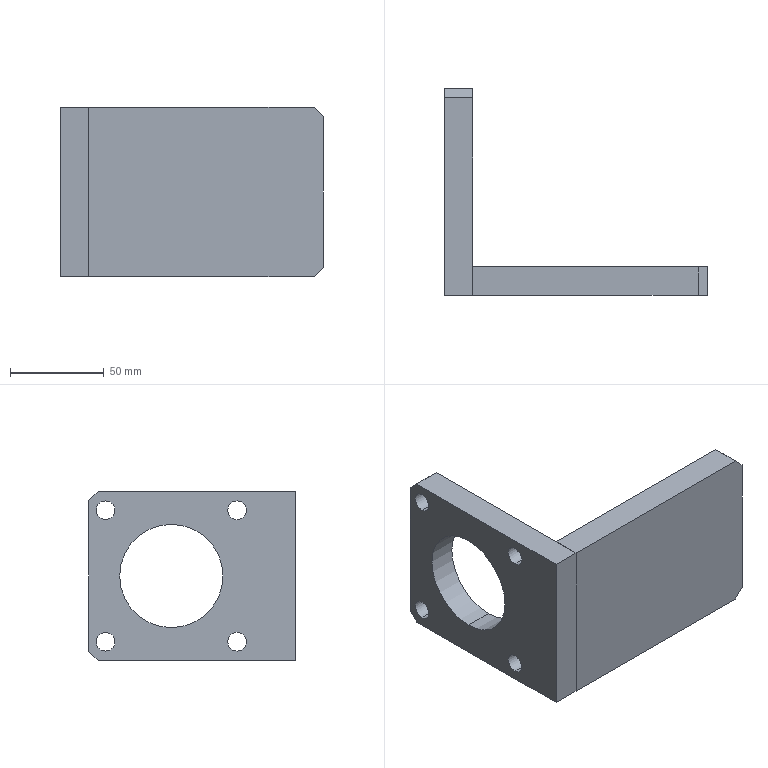Part | STEP file | Hydraulic Cylinder Fixing Bracket | 2 solids | 46 faces | box 140 x 110 x 90 mm | volume 268205 mm3 | plane 28 | cylinder 18 | commonest cylinder face diameters 9 x8 10 x8 55 x2
STEP:
#1=CARTESIAN_POINT('',(-38.428,-20.407,0.));
#2=VERTEX_POINT('',#1);
#3=CARTESIAN_POINT('',(81.572,-20.407,0.));
#4=VERTEX_POINT('',#3);
#5=CARTESIAN_POINT('',(-38.428,-20.407,0.));
#6=DIRECTION('',(1.,0.,0.));
#7=VECTOR('',#6,1000.);
#8=LINE('',#5,#7);
#9=EDGE_CURVE('',#2,#4,#8,.T.);
#10=ORIENTED_EDGE('',*,*,#9,.T.);
#11=CARTESIAN_POINT('',(86.572,-20.407,5.));
#12=VERTEX_POINT('',#11);
#13=CARTESIAN_POINT('',(81.572,-20.407,0.));
#14=DIRECTION('',(0.7071,0.,0.7071));
#15=VECTOR('',#14,1000.);
#16=LINE('',#13,#15);
#17=EDGE_CURVE('',#4,#12,#16,.T.);
#18=ORIENTED_EDGE('',*,*,#17,.T.);
#19=CARTESIAN_POINT('',(86.572,-20.407,85.));
#20=VERTEX_POINT('',#19);
#21=CARTESIAN_POINT('',(86.572,-20.407,-125.897));
#22=DIRECTION('',(0.,0.,1.));
#23=VECTOR('',#22,1000.);
#24=LINE('',#21,#23);
#25=EDGE_CURVE('',#12,#20,#24,.T.);
#26=ORIENTED_EDGE('',*,*,#25,.T.);
#27=CARTESIAN_POINT('',(81.572,-20.407,90.));
#28=VERTEX_POINT('',#27);
#29=CARTESIAN_POINT('',(86.572,-20.407,85.));
#30=DIRECTION('',(-0.7071,0.,0.7071));
#31=VECTOR('',#30,1000.);
#32=LINE('',#29,#31);
#33=EDGE_CURVE('',#20,#28,#32,.T.);
#34=ORIENTED_EDGE('',*,*,#33,.T.);
#35=CARTESIAN_POINT('',(-38.428,-20.407,90.));
#36=VERTEX_POINT('',#35);
#37=CARTESIAN_POINT('',(-38.428,-20.407,90.));
#38=DIRECTION('',(-1.,0.,0.));
#39=VECTOR('',#38,1000.);
#40=LINE('',#37,#39);
#41=EDGE_CURVE('',#28,#36,#40,.T.);
#42=ORIENTED_EDGE('',*,*,#41,.T.);
#43=CARTESIAN_POINT('',(-38.428,-20.407,-125.897));
#44=DIRECTION('',(0.,0.,-1.));
#45=VECTOR('',#44,1000.);
#46=LINE('',#43,#45);
#47=EDGE_CURVE('',#36,#2,#46,.T.);
#48=ORIENTED_EDGE('',*,*,#47,.T.);
#49=EDGE_LOOP('',(#10,#18,#26,#34,#42,#48));
#50=FACE_OUTER_BOUND('',#49,.T.);
#51=CARTESIAN_POINT('',(-38.428,-20.407,-125.897));
#52=DIRECTION('',(0.,-1.,0.));
#53=DIRECTION('',(0.,0.,-1.));
#54=AXIS2_PLACEMENT_3D('',#51,#52,#53);
#55=PLANE('',#54);
#56=ADVANCED_FACE('',(#50),#55,.T.);
#57=CARTESIAN_POINT('',(81.572,-5.407,0.));
#58=VERTEX_POINT('',#57);
#59=CARTESIAN_POINT('',(81.572,-20.407,0.));
#60=DIRECTION('',(0.,-1.,0.));
#61=VECTOR('',#60,1000.);
#62=LINE('',#59,#61);
#63=EDGE_CURVE('',#58,#4,#62,.T.);
#64=ORIENTED_EDGE('',*,*,#63,.F.);
#65=CARTESIAN_POINT('',(86.572,-5.407,5.));
#66=VERTEX_POINT('',#65);
#67=CARTESIAN_POINT('',(86.572,-5.407,5.));
#68=DIRECTION('',(-0.7071,0.,-0.7071));
#69=VECTOR('',#68,1000.);
#70=LINE('',#67,#69);
#71=EDGE_CURVE('',#66,#58,#70,.T.);
#72=ORIENTED_EDGE('',*,*,#71,.F.);
#73=CARTESIAN_POINT('',(86.572,-20.407,5.));
#74=DIRECTION('',(0.,1.,0.));
#75=VECTOR('',#74,1000.);
#76=LINE('',#73,#75);
#77=EDGE_CURVE('',#12,#66,#76,.T.);
#78=ORIENTED_EDGE('',*,*,#77,.F.);
#79=ORIENTED_EDGE('',*,*,#17,.F.);
#80=EDGE_LOOP('',(#64,#72,#78,#79));
#81=FACE_OUTER_BOUND('',#80,.T.);
#82=CARTESIAN_POINT('',(86.572,-20.407,5.));
#83=DIRECTION('',(-0.7071,0.,0.7071));
#84=DIRECTION('',(0.7071,0.,0.7071));
#85=AXIS2_PLACEMENT_3D('',#82,#83,#84);
#86=PLANE('',#85);
#87=ADVANCED_FACE('',(#81),#86,.F.);
#88=ORIENTED_EDGE('',*,*,#9,.F.);
#89=CARTESIAN_POINT('',(-38.428,-5.407,0.));
#90=VERTEX_POINT('',#89);
#91=CARTESIAN_POINT('',(-38.428,0.,0.));
#92=DIRECTION('',(0.,1.,0.));
#93=VECTOR('',#92,1000.);
#94=LINE('',#91,#93);
#95=EDGE_CURVE('',#2,#90,#94,.T.);
#96=ORIENTED_EDGE('',*,*,#95,.T.);
#97=CARTESIAN_POINT('',(0.,-5.407,0.));
#98=DIRECTION('',(1.,0.,0.));
#99=VECTOR('',#98,1000.);
#100=LINE('',#97,#99);
#101=EDGE_CURVE('',#90,#58,#100,.T.);
#102=ORIENTED_EDGE('',*,*,#101,.T.);
#103=ORIENTED_EDGE('',*,*,#63,.T.);
#104=EDGE_LOOP('',(#88,#96,#102,#103));
#105=FACE_OUTER_BOUND('',#104,.T.);
#106=CARTESIAN_POINT('',(0.,0.,0.));
#107=DIRECTION('',(0.,0.,-1.));
#108=DIRECTION('',(-1.,0.,0.));
#109=AXIS2_PLACEMENT_3D('',#106,#107,#108);
#110=PLANE('',#109);
#111=ADVANCED_FACE('',(#105),#110,.T.);
#112=ORIENTED_EDGE('',*,*,#47,.F.);
#113=CARTESIAN_POINT('',(-38.428,-5.407,90.));
#114=VERTEX_POINT('',#113);
#115=CARTESIAN_POINT('',(-38.428,-20.407,90.));
#116=DIRECTION('',(0.,1.,0.));
#117=VECTOR('',#116,1000.);
#118=LINE('',#115,#117);
#119=EDGE_CURVE('',#36,#114,#118,.T.);
#120=ORIENTED_EDGE('',*,*,#119,.T.);
#121=CARTESIAN_POINT('',(-38.428,-5.407,-125.897));
#122=DIRECTION('',(0.,0.,-1.));
#123=VECTOR('',#122,1000.);
#124=LINE('',#121,#123);
#125=EDGE_CURVE('',#114,#90,#124,.T.);
#126=ORIENTED_EDGE('',*,*,#125,.T.);
#127=ORIENTED_EDGE('',*,*,#95,.F.);
#128=EDGE_LOOP('',(#112,#120,#126,#127));
#129=FACE_OUTER_BOUND('',#128,.T.);
#130=CARTESIAN_POINT('',(-38.428,-20.407,-125.897));
#131=DIRECTION('',(-1.,0.,0.));
#132=DIRECTION('',(0.,0.,1.));
#133=AXIS2_PLACEMENT_3D('',#130,#131,#132);
#134=PLANE('',#133);
#135=ADVANCED_FACE('',(#129),#134,.T.);
#136=CARTESIAN_POINT('',(81.572,-5.407,90.));
#137=VERTEX_POINT('',#136);
#138=CARTESIAN_POINT('',(81.572,0.,90.));
#139=DIRECTION('',(0.,-1.,0.));
#140=VECTOR('',#139,1000.);
#141=LINE('',#138,#140);
#142=EDGE_CURVE('',#137,#28,#141,.T.);
#143=ORIENTED_EDGE('',*,*,#142,.F.);
#144=CARTESIAN_POINT('',(0.,-5.407,90.));
#145=DIRECTION('',(1.,0.,0.));
#146=VECTOR('',#145,1000.);
#147=LINE('',#144,#146);
#148=EDGE_CURVE('',#114,#137,#147,.T.);
#149=ORIENTED_EDGE('',*,*,#148,.F.);
#150=ORIENTED_EDGE('',*,*,#119,.F.);
#151=ORIENTED_EDGE('',*,*,#41,.F.);
#152=EDGE_LOOP('',(#143,#149,#150,#151));
#153=FACE_OUTER_BOUND('',#152,.T.);
#154=CARTESIAN_POINT('',(0.,0.,90.));
#155=DIRECTION('',(0.,0.,-1.));
#156=DIRECTION('',(-1.,0.,0.));
#157=AXIS2_PLACEMENT_3D('',#154,#155,#156);
#158=PLANE('',#157);
#159=ADVANCED_FACE('',(#153),#158,.F.);
#160=CARTESIAN_POINT('',(86.572,-5.407,85.));
#161=VERTEX_POINT('',#160);
#162=CARTESIAN_POINT('',(81.572,-5.407,90.));
#163=DIRECTION('',(-0.7071,0.,0.7071));
#164=VECTOR('',#163,1000.);
#165=LINE('',#162,#164);
#166=EDGE_CURVE('',#161,#137,#165,.T.);
#167=ORIENTED_EDGE('',*,*,#166,.T.);
#168=ORIENTED_EDGE('',*,*,#142,.T.);
#169=ORIENTED_EDGE('',*,*,#33,.F.);
#170=CARTESIAN_POINT('',(86.572,0.,85.));
#171=DIRECTION('',(0.,1.,0.));
#172=VECTOR('',#171,1000.);
#173=LINE('',#170,#172);
#174=EDGE_CURVE('',#20,#161,#173,.T.);
#175=ORIENTED_EDGE('',*,*,#174,.T.);
#176=EDGE_LOOP('',(#167,#168,#169,#175));
#177=FACE_OUTER_BOUND('',#176,.T.);
#178=CARTESIAN_POINT('',(81.572,0.,90.));
#179=DIRECTION('',(0.7071,0.,0.7071));
#180=DIRECTION('',(0.7071,0.,-0.7071));
#181=AXIS2_PLACEMENT_3D('',#178,#179,#180);
#182=PLANE('',#181);
#183=ADVANCED_FACE('',(#177),#182,.T.);
#184=ORIENTED_EDGE('',*,*,#25,.F.);
#185=ORIENTED_EDGE('',*,*,#77,.T.);
#186=CARTESIAN_POINT('',(86.572,-5.407,-125.897));
#187=DIRECTION('',(0.,0.,1.));
#188=VECTOR('',#187,1000.);
#189=LINE('',#186,#188);
#190=EDGE_CURVE('',#66,#161,#189,.T.);
#191=ORIENTED_EDGE('',*,*,#190,.T.);
#192=ORIENTED_EDGE('',*,*,#174,.F.);
#193=EDGE_LOOP('',(#184,#185,#191,#192));
#194=FACE_OUTER_BOUND('',#193,.T.);
#195=CARTESIAN_POINT('',(86.572,-20.407,-125.897));
#196=DIRECTION('',(1.,0.,0.));
#197=DIRECTION('',(0.,1.,0.));
#198=AXIS2_PLACEMENT_3D('',#195,#196,#197);
#199=PLANE('',#198);
#200=ADVANCED_FACE('',(#194),#199,.T.);
#201=ORIENTED_EDGE('',*,*,#101,.F.);
#202=ORIENTED_EDGE('',*,*,#125,.F.);
#203=ORIENTED_EDGE('',*,*,#148,.T.);
#204=ORIENTED_EDGE('',*,*,#166,.F.);
#205=ORIENTED_EDGE('',*,*,#190,.F.);
#206=ORIENTED_EDGE('',*,*,#71,.T.);
#207=EDGE_LOOP('',(#201,#202,#203,#204,#205,#206));
#208=FACE_OUTER_BOUND('',#207,.T.);
#209=CARTESIAN_POINT('',(19.072,-5.407,7.5));
#210=VERTEX_POINT('',#209);
#211=CARTESIAN_POINT('',(19.072,-5.407,16.5));
#212=VERTEX_POINT('',#211);
#213=CARTESIAN_POINT('',(19.072,-5.407,12.));
#214=DIRECTION('',(0.,-1.,0.));
#215=DIRECTION('',(0.,0.,1.));
#216=AXIS2_PLACEMENT_3D('',#213,#214,#215);
#217=CIRCLE('',#216,4.5);
#218=EDGE_CURVE('',#210,#212,#217,.T.);
#219=ORIENTED_EDGE('',*,*,#218,.T.);
#220=CARTESIAN_POINT('',(4.072,-5.407,16.5));
#221=VERTEX_POINT('',#220);
#222=CARTESIAN_POINT('',(-38.428,-5.407,16.5));
#223=DIRECTION('',(-1.,0.,0.));
#224=VECTOR('',#223,1000.);
#225=LINE('',#222,#224);
#226=EDGE_CURVE('',#212,#221,#225,.T.);
#227=ORIENTED_EDGE('',*,*,#226,.T.);
#228=CARTESIAN_POINT('',(4.072,-5.407,7.5));
#229=VERTEX_POINT('',#228);
#230=CARTESIAN_POINT('',(4.072,-5.407,12.));
#231=DIRECTION('',(0.,-1.,0.));
#232=DIRECTION('',(0.,0.,1.));
#233=AXIS2_PLACEMENT_3D('',#230,#231,#232);
#234=CIRCLE('',#233,4.5);
#235=EDGE_CURVE('',#221,#229,#234,.T.);
#236=ORIENTED_EDGE('',*,*,#235,.T.);
#237=CARTESIAN_POINT('',(-38.428,-5.407,7.5));
#238=DIRECTION('',(1.,0.,0.));
#239=VECTOR('',#238,1000.);
#240=LINE('',#237,#239);
#241=EDGE_CURVE('',#229,#210,#240,.T.);
#242=ORIENTED_EDGE('',*,*,#241,.T.);
#243=EDGE_LOOP('',(#219,#227,#236,#242));
#244=FACE_BOUND('',#243,.T.);
#245=CARTESIAN_POINT('',(69.072,-5.407,7.5));
#246=VERTEX_POINT('',#245);
#247=CARTESIAN_POINT('',(69.072,-5.407,16.5));
#248=VERTEX_POINT('',#247);
#249=CARTESIAN_POINT('',(69.072,-5.407,12.));
#250=DIRECTION('',(0.,-1.,0.));
#251=DIRECTION('',(0.,0.,1.));
#252=AXIS2_PLACEMENT_3D('',#249,#250,#251);
#253=CIRCLE('',#252,4.5);
#254=EDGE_CURVE('',#246,#248,#253,.T.);
#255=ORIENTED_EDGE('',*,*,#254,.T.);
#256=CARTESIAN_POINT('',(54.072,-5.407,16.5));
#257=VERTEX_POINT('',#256);
#258=CARTESIAN_POINT('',(-38.428,-5.407,16.5));
#259=DIRECTION('',(-1.,0.,0.));
#260=VECTOR('',#259,1000.);
#261=LINE('',#258,#260);
#262=EDGE_CURVE('',#248,#257,#261,.T.);
#263=ORIENTED_EDGE('',*,*,#262,.T.);
#264=CARTESIAN_POINT('',(54.072,-5.407,7.5));
#265=VERTEX_POINT('',#264);
#266=CARTESIAN_POINT('',(54.072,-5.407,12.));
#267=DIRECTION('',(0.,-1.,0.));
#268=DIRECTION('',(0.,0.,1.));
#269=AXIS2_PLACEMENT_3D('',#266,#267,#268);
#270=CIRCLE('',#269,4.5);
#271=EDGE_CURVE('',#257,#265,#270,.T.);
#272=ORIENTED_EDGE('',*,*,#271,.T.);
#273=CARTESIAN_POINT('',(-38.428,-5.407,7.5));
#274=DIRECTION('',(1.,0.,0.));
#275=VECTOR('',#274,1000.);
#276=LINE('',#273,#275);
#277=EDGE_CURVE('',#265,#246,#276,.T.);
#278=ORIENTED_EDGE('',*,*,#277,.T.);
#279=EDGE_LOOP('',(#255,#263,#272,#278));
#280=FACE_BOUND('',#279,.T.);
#281=CARTESIAN_POINT('',(69.072,-5.407,73.5));
#282=VERTEX_POINT('',#281);
#283=CARTESIAN_POINT('',(69.072,-5.407,82.5));
#284=VERTEX_POINT('',#283);
#285=CARTESIAN_POINT('',(69.072,-5.407,78.));
#286=DIRECTION('',(0.,-1.,0.));
#287=DIRECTION('',(0.,0.,1.));
#288=AXIS2_PLACEMENT_3D('',#285,#286,#287);
#289=CIRCLE('',#288,4.5);
#290=EDGE_CURVE('',#282,#284,#289,.T.);
#291=ORIENTED_EDGE('',*,*,#290,.T.);
#292=CARTESIAN_POINT('',(54.072,-5.407,82.5));
#293=VERTEX_POINT('',#292);
#294=CARTESIAN_POINT('',(-38.428,-5.407,82.5));
#295=DIRECTION('',(-1.,0.,0.));
#296=VECTOR('',#295,1000.);
#297=LINE('',#294,#296);
#298=EDGE_CURVE('',#284,#293,#297,.T.);
#299=ORIENTED_EDGE('',*,*,#298,.T.);
#300=CARTESIAN_POINT('',(54.072,-5.407,73.5));
#301=VERTEX_POINT('',#300);
#302=CARTESIAN_POINT('',(54.072,-5.407,78.));
#303=DIRECTION('',(0.,-1.,0.));
#304=DIRECTION('',(0.,0.,1.));
#305=AXIS2_PLACEMENT_3D('',#302,#303,#304);
#306=CIRCLE('',#305,4.5);
#307=EDGE_CURVE('',#293,#301,#306,.T.);
#308=ORIENTED_EDGE('',*,*,#307,.T.);
#309=CARTESIAN_POINT('',(-38.428,-5.407,73.5));
#310=DIRECTION('',(1.,0.,0.));
#311=VECTOR('',#310,1000.);
#312=LINE('',#309,#311);
#313=EDGE_CURVE('',#301,#282,#312,.T.);
#314=ORIENTED_EDGE('',*,*,#313,.T.);
#315=EDGE_LOOP('',(#291,#299,#308,#314));
#316=FACE_BOUND('',#315,.T.);
#317=CARTESIAN_POINT('',(19.072,-5.407,73.5));
#318=VERTEX_POINT('',#317);
#319=CARTESIAN_POINT('',(19.072,-5.407,82.5));
#320=VERTEX_POINT('',#319);
#321=CARTESIAN_POINT('',(19.072,-5.407,78.));
#322=DIRECTION('',(0.,-1.,0.));
#323=DIRECTION('',(0.,0.,1.));
#324=AXIS2_PLACEMENT_3D('',#321,#322,#323);
#325=CIRCLE('',#324,4.5);
#326=EDGE_CURVE('',#318,#320,#325,.T.);
#327=ORIENTED_EDGE('',*,*,#326,.T.);
#328=CARTESIAN_POINT('',(4.072,-5.407,82.5));
#329=VERTEX_POINT('',#328);
#330=CARTESIAN_POINT('',(-38.428,-5.407,82.5));
#331=DIRECTION('',(-1.,0.,0.));
#332=VECTOR('',#331,1000.);
#333=LINE('',#330,#332);
#334=EDGE_CURVE('',#320,#329,#333,.T.);
#335=ORIENTED_EDGE('',*,*,#334,.T.);
#336=CARTESIAN_POINT('',(4.072,-5.407,73.5));
#337=VERTEX_POINT('',#336);
#338=CARTESIAN_POINT('',(4.072,-5.407,78.));
#339=DIRECTION('',(0.,-1.,0.));
#340=DIRECTION('',(0.,0.,1.));
#341=AXIS2_PLACEMENT_3D('',#338,#339,#340);
#342=CIRCLE('',#341,4.5);
#343=EDGE_CURVE('',#329,#337,#342,.T.);
#344=ORIENTED_EDGE('',*,*,#343,.T.);
#345=CARTESIAN_POINT('',(-38.428,-5.407,73.5));
#346=DIRECTION('',(1.,0.,0.));
#347=VECTOR('',#346,1000.);
#348=LINE('',#345,#347);
#349=EDGE_CURVE('',#337,#318,#348,.T.);
#350=ORIENTED_EDGE('',*,*,#349,.T.);
#351=EDGE_LOOP('',(#327,#335,#344,#350));
#352=FACE_BOUND('',#351,.T.);
#353=CARTESIAN_POINT('',(-38.428,-5.407,-125.897));
#354=DIRECTION('',(0.,1.,0.));
#355=DIRECTION('',(0.,0.,1.));
#356=AXIS2_PLACEMENT_3D('',#353,#354,#355);
#357=PLANE('',#356);
#358=ADVANCED_FACE('',(#208,#244,#280,#316,#352),#357,.T.);
#359=CARTESIAN_POINT('',(19.072,-15.407,16.5));
#360=VERTEX_POINT('',#359);
#361=CARTESIAN_POINT('',(19.072,-15.407,16.5));
#362=DIRECTION('',(0.,1.,0.));
#363=VECTOR('',#362,1000.);
#364=LINE('',#361,#363);
#365=EDGE_CURVE('',#360,#212,#364,.T.);
#366=ORIENTED_EDGE('',*,*,#365,.F.);
#367=CARTESIAN_POINT('',(4.072,-15.407,16.5));
#368=VERTEX_POINT('',#367);
#369=CARTESIAN_POINT('',(4.072,-15.407,16.5));
#370=DIRECTION('',(1.,0.,0.));
#371=VECTOR('',#370,1000.);
#372=LINE('',#369,#371);
#373=EDGE_CURVE('',#368,#360,#372,.T.);
#374=ORIENTED_EDGE('',*,*,#373,.F.);
#375=CARTESIAN_POINT('',(4.072,-15.407,16.5));
#376=DIRECTION('',(0.,-1.,0.));
#377=VECTOR('',#376,1000.);
#378=LINE('',#375,#377);
#379=EDGE_CURVE('',#221,#368,#378,.T.);
#380=ORIENTED_EDGE('',*,*,#379,.F.);
#381=ORIENTED_EDGE('',*,*,#226,.F.);
#382=EDGE_LOOP('',(#366,#374,#380,#381));
#383=FACE_OUTER_BOUND('',#382,.T.);
#384=CARTESIAN_POINT('',(4.072,-15.407,16.5));
#385=DIRECTION('',(0.,0.,1.));
#386=DIRECTION('',(1.,0.,0.));
#387=AXIS2_PLACEMENT_3D('',#384,#385,#386);
#388=PLANE('',#387);
#389=ADVANCED_FACE('',(#383),#388,.F.);
#390=CARTESIAN_POINT('',(19.072,-15.407,7.5));
#391=VERTEX_POINT('',#390);
#392=CARTESIAN_POINT('',(19.072,-15.407,7.5));
#393=DIRECTION('',(0.,1.,0.));
#394=VECTOR('',#393,1000.);
#395=LINE('',#392,#394);
#396=EDGE_CURVE('',#391,#210,#395,.T.);
#397=ORIENTED_EDGE('',*,*,#396,.F.);
#398=CARTESIAN_POINT('',(19.072,-15.407,12.));
#399=DIRECTION('',(0.,1.,0.));
#400=DIRECTION('',(0.,0.,1.));
#401=AXIS2_PLACEMENT_3D('',#398,#399,#400);
#402=CIRCLE('',#401,4.5);
#403=EDGE_CURVE('',#360,#391,#402,.T.);
#404=ORIENTED_EDGE('',*,*,#403,.F.);
#405=ORIENTED_EDGE('',*,*,#365,.T.);
#406=ORIENTED_EDGE('',*,*,#218,.F.);
#407=EDGE_LOOP('',(#397,#404,#405,#406));
#408=FACE_OUTER_BOUND('',#407,.T.);
#409=CARTESIAN_POINT('',(19.072,-15.407,12.));
#410=DIRECTION('',(0.,1.,0.));
#411=DIRECTION('',(0.,0.,1.));
#412=AXIS2_PLACEMENT_3D('',#409,#410,#411);
#413=CYLINDRICAL_SURFACE('',#412,4.5);
#414=ADVANCED_FACE('',(#408),#413,.F.);
#415=CARTESIAN_POINT('',(4.072,-15.407,7.5));
#416=VERTEX_POINT('',#415);
#417=CARTESIAN_POINT('',(4.072,-15.407,7.5));
#418=DIRECTION('',(0.,1.,0.));
#419=VECTOR('',#418,1000.);
#420=LINE('',#417,#419);
#421=EDGE_CURVE('',#416,#229,#420,.T.);
#422=ORIENTED_EDGE('',*,*,#421,.F.);
#423=CARTESIAN_POINT('',(4.072,-15.407,7.5));
#424=DIRECTION('',(-1.,0.,0.));
#425=VECTOR('',#424,1000.);
#426=LINE('',#423,#425);
#427=EDGE_CURVE('',#391,#416,#426,.T.);
#428=ORIENTED_EDGE('',*,*,#427,.F.);
#429=ORIENTED_EDGE('',*,*,#396,.T.);
#430=ORIENTED_EDGE('',*,*,#241,.F.);
#431=EDGE_LOOP('',(#422,#428,#429,#430));
#432=FACE_OUTER_BOUND('',#431,.T.);
#433=CARTESIAN_POINT('',(4.072,-15.407,7.5));
#434=DIRECTION('',(0.,0.,-1.));
#435=DIRECTION('',(-1.,0.,0.));
#436=AXIS2_PLACEMENT_3D('',#433,#434,#435);
#437=PLANE('',#436);
#438=ADVANCED_FACE('',(#432),#437,.F.);
#439=ORIENTED_EDGE('',*,*,#379,.T.);
#440=CARTESIAN_POINT('',(4.072,-15.407,12.));
#441=DIRECTION('',(0.,1.,0.));
#442=DIRECTION('',(0.,0.,1.));
#443=AXIS2_PLACEMENT_3D('',#440,#441,#442);
#444=CIRCLE('',#443,4.5);
#445=EDGE_CURVE('',#416,#368,#444,.T.);
#446=ORIENTED_EDGE('',*,*,#445,.F.);
#447=ORIENTED_EDGE('',*,*,#421,.T.);
#448=ORIENTED_EDGE('',*,*,#235,.F.);
#449=EDGE_LOOP('',(#439,#446,#447,#448));
#450=FACE_OUTER_BOUND('',#449,.T.);
#451=CARTESIAN_POINT('',(4.072,-15.407,12.));
#452=DIRECTION('',(0.,1.,0.));
#453=DIRECTION('',(0.,0.,1.));
#454=AXIS2_PLACEMENT_3D('',#451,#452,#453);
#455=CYLINDRICAL_SURFACE('',#454,4.5);
#456=ADVANCED_FACE('',(#450),#455,.F.);
#457=CARTESIAN_POINT('',(69.072,-15.407,16.5));
#458=VERTEX_POINT('',#457);
#459=CARTESIAN_POINT('',(69.072,-15.407,16.5));
#460=DIRECTION('',(0.,1.,0.));
#461=VECTOR('',#460,1000.);
#462=LINE('',#459,#461);
#463=EDGE_CURVE('',#458,#248,#462,.T.);
#464=ORIENTED_EDGE('',*,*,#463,.F.);
#465=CARTESIAN_POINT('',(54.072,-15.407,16.5));
#466=VERTEX_POINT('',#465);
#467=CARTESIAN_POINT('',(54.072,-15.407,16.5));
#468=DIRECTION('',(1.,0.,0.));
#469=VECTOR('',#468,1000.);
#470=LINE('',#467,#469);
#471=EDGE_CURVE('',#466,#458,#470,.T.);
#472=ORIENTED_EDGE('',*,*,#471,.F.);
#473=CARTESIAN_POINT('',(54.072,-15.407,16.5));
#474=DIRECTION('',(0.,-1.,0.));
#475=VECTOR('',#474,1000.);
#476=LINE('',#473,#475);
#477=EDGE_CURVE('',#257,#466,#476,.T.);
#478=ORIENTED_EDGE('',*,*,#477,.F.);
#479=ORIENTED_EDGE('',*,*,#262,.F.);
#480=EDGE_LOOP('',(#464,#472,#478,#479));
#481=FACE_OUTER_BOUND('',#480,.T.);
#482=CARTESIAN_POINT('',(54.072,-15.407,16.5));
#483=DIRECTION('',(0.,0.,1.));
#484=DIRECTION('',(1.,0.,0.));
#485=AXIS2_PLACEMENT_3D('',#482,#483,#484);
#486=PLANE('',#485);
#487=ADVANCED_FACE('',(#481),#486,.F.);
#488=CARTESIAN_POINT('',(69.072,-15.407,7.5));
#489=VERTEX_POINT('',#488);
#490=CARTESIAN_POINT('',(69.072,-15.407,7.5));
#491=DIRECTION('',(0.,1.,0.));
#492=VECTOR('',#491,1000.);
#493=LINE('',#490,#492);
#494=EDGE_CURVE('',#489,#246,#493,.T.);
#495=ORIENTED_EDGE('',*,*,#494,.F.);
#496=CARTESIAN_POINT('',(69.072,-15.407,12.));
#497=DIRECTION('',(0.,1.,0.));
#498=DIRECTION('',(0.,0.,1.));
#499=AXIS2_PLACEMENT_3D('',#496,#497,#498);
#500=CIRCLE('',#499,4.5);
#501=EDGE_CURVE('',#458,#489,#500,.T.);
#502=ORIENTED_EDGE('',*,*,#501,.F.);
#503=ORIENTED_EDGE('',*,*,#463,.T.);
#504=ORIENTED_EDGE('',*,*,#254,.F.);
#505=EDGE_LOOP('',(#495,#502,#503,#504));
#506=FACE_OUTER_BOUND('',#505,.T.);
#507=CARTESIAN_POINT('',(69.072,-15.407,12.));
#508=DIRECTION('',(0.,1.,0.));
#509=DIRECTION('',(0.,0.,1.));
#510=AXIS2_PLACEMENT_3D('',#507,#508,#509);
#511=CYLINDRICAL_SURFACE('',#510,4.5);
#512=ADVANCED_FACE('',(#506),#511,.F.);
#513=CARTESIAN_POINT('',(54.072,-15.407,7.5));
#514=VERTEX_POINT('',#513);
#515=CARTESIAN_POINT('',(54.072,-15.407,7.5));
#516=DIRECTION('',(0.,1.,0.));
#517=VECTOR('',#516,1000.);
#518=LINE('',#515,#517);
#519=EDGE_CURVE('',#514,#265,#518,.T.);
#520=ORIENTED_EDGE('',*,*,#519,.F.);
#521=CARTESIAN_POINT('',(54.072,-15.407,7.5));
#522=DIRECTION('',(-1.,0.,0.));
#523=VECTOR('',#522,1000.);
#524=LINE('',#521,#523);
#525=EDGE_CURVE('',#489,#514,#524,.T.);
#526=ORIENTED_EDGE('',*,*,#525,.F.);
#527=ORIENTED_EDGE('',*,*,#494,.T.);
#528=ORIENTED_EDGE('',*,*,#277,.F.);
#529=EDGE_LOOP('',(#520,#526,#527,#528));
#530=FACE_OUTER_BOUND('',#529,.T.);
#531=CARTESIAN_POINT('',(54.072,-15.407,7.5));
#532=DIRECTION('',(0.,0.,-1.));
#533=DIRECTION('',(-1.,0.,0.));
#534=AXIS2_PLACEMENT_3D('',#531,#532,#533);
#535=PLANE('',#534);
#536=ADVANCED_FACE('',(#530),#535,.F.);
#537=ORIENTED_EDGE('',*,*,#477,.T.);
#538=CARTESIAN_POINT('',(54.072,-15.407,12.));
#539=DIRECTION('',(0.,1.,0.));
#540=DIRECTION('',(0.,0.,1.));
#541=AXIS2_PLACEMENT_3D('',#538,#539,#540);
#542=CIRCLE('',#541,4.5);
#543=EDGE_CURVE('',#514,#466,#542,.T.);
#544=ORIENTED_EDGE('',*,*,#543,.F.);
#545=ORIENTED_EDGE('',*,*,#519,.T.);
#546=ORIENTED_EDGE('',*,*,#271,.F.);
#547=EDGE_LOOP('',(#537,#544,#545,#546));
#548=FACE_OUTER_BOUND('',#547,.T.);
#549=CARTESIAN_POINT('',(54.072,-15.407,12.));
#550=DIRECTION('',(0.,1.,0.));
#551=DIRECTION('',(0.,0.,1.));
#552=AXIS2_PLACEMENT_3D('',#549,#550,#551);
#553=CYLINDRICAL_SURFACE('',#552,4.5);
#554=ADVANCED_FACE('',(#548),#553,.F.);
#555=CARTESIAN_POINT('',(69.072,-15.407,82.5));
#556=VERTEX_POINT('',#555);
#557=CARTESIAN_POINT('',(69.072,-15.407,82.5));
#558=DIRECTION('',(0.,1.,0.));
#559=VECTOR('',#558,1000.);
#560=LINE('',#557,#559);
#561=EDGE_CURVE('',#556,#284,#560,.T.);
#562=ORIENTED_EDGE('',*,*,#561,.F.);
#563=CARTESIAN_POINT('',(54.072,-15.407,82.5));
#564=VERTEX_POINT('',#563);
#565=CARTESIAN_POINT('',(54.072,-15.407,82.5));
#566=DIRECTION('',(1.,0.,0.));
#567=VECTOR('',#566,1000.);
#568=LINE('',#565,#567);
#569=EDGE_CURVE('',#564,#556,#568,.T.);
#570=ORIENTED_EDGE('',*,*,#569,.F.);
#571=CARTESIAN_POINT('',(54.072,-15.407,82.5));
#572=DIRECTION('',(0.,-1.,0.));
#573=VECTOR('',#572,1000.);
#574=LINE('',#571,#573);
#575=EDGE_CURVE('',#293,#564,#574,.T.);
#576=ORIENTED_EDGE('',*,*,#575,.F.);
#577=ORIENTED_EDGE('',*,*,#298,.F.);
#578=EDGE_LOOP('',(#562,#570,#576,#577));
#579=FACE_OUTER_BOUND('',#578,.T.);
#580=CARTESIAN_POINT('',(54.072,-15.407,82.5));
#581=DIRECTION('',(0.,0.,1.));
#582=DIRECTION('',(1.,0.,0.));
#583=AXIS2_PLACEMENT_3D('',#580,#581,#582);
#584=PLANE('',#583);
#585=ADVANCED_FACE('',(#579),#584,.F.);
#586=CARTESIAN_POINT('',(69.072,-15.407,73.5));
#587=VERTEX_POINT('',#586);
#588=CARTESIAN_POINT('',(69.072,-15.407,73.5));
#589=DIRECTION('',(0.,1.,0.));
#590=VECTOR('',#589,1000.);
#591=LINE('',#588,#590);
#592=EDGE_CURVE('',#587,#282,#591,.T.);
#593=ORIENTED_EDGE('',*,*,#592,.F.);
#594=CARTESIAN_POINT('',(69.072,-15.407,78.));
#595=DIRECTION('',(0.,1.,0.));
#596=DIRECTION('',(0.,0.,1.));
#597=AXIS2_PLACEMENT_3D('',#594,#595,#596);
#598=CIRCLE('',#597,4.5);
#599=EDGE_CURVE('',#556,#587,#598,.T.);
#600=ORIENTED_EDGE('',*,*,#599,.F.);
#601=ORIENTED_EDGE('',*,*,#561,.T.);
#602=ORIENTED_EDGE('',*,*,#290,.F.);
#603=EDGE_LOOP('',(#593,#600,#601,#602));
#604=FACE_OUTER_BOUND('',#603,.T.);
#605=CARTESIAN_POINT('',(69.072,-15.407,78.));
#606=DIRECTION('',(0.,1.,0.));
#607=DIRECTION('',(0.,0.,1.));
#608=AXIS2_PLACEMENT_3D('',#605,#606,#607);
#609=CYLINDRICAL_SURFACE('',#608,4.5);
#610=ADVANCED_FACE('',(#604),#609,.F.);
#611=CARTESIAN_POINT('',(54.072,-15.407,73.5));
#612=VERTEX_POINT('',#611);
#613=CARTESIAN_POINT('',(54.072,-15.407,73.5));
#614=DIRECTION('',(0.,1.,0.));
#615=VECTOR('',#614,1000.);
#616=LINE('',#613,#615);
#617=EDGE_CURVE('',#612,#301,#616,.T.);
#618=ORIENTED_EDGE('',*,*,#617,.F.);
#619=CARTESIAN_POINT('',(54.072,-15.407,73.5));
#620=DIRECTION('',(-1.,0.,0.));
#621=VECTOR('',#620,1000.);
#622=LINE('',#619,#621);
#623=EDGE_CURVE('',#587,#612,#622,.T.);
#624=ORIENTED_EDGE('',*,*,#623,.F.);
#625=ORIENTED_EDGE('',*,*,#592,.T.);
#626=ORIENTED_EDGE('',*,*,#313,.F.);
#627=EDGE_LOOP('',(#618,#624,#625,#626));
#628=FACE_OUTER_BOUND('',#627,.T.);
#629=CARTESIAN_POINT('',(54.072,-15.407,73.5));
#630=DIRECTION('',(0.,0.,-1.));
#631=DIRECTION('',(-1.,0.,0.));
#632=AXIS2_PLACEMENT_3D('',#629,#630,#631);
#633=PLANE('',#632);
#634=ADVANCED_FACE('',(#628),#633,.F.);
#635=ORIENTED_EDGE('',*,*,#575,.T.);
#636=CARTESIAN_POINT('',(54.072,-15.407,78.));
#637=DIRECTION('',(0.,1.,0.));
#638=DIRECTION('',(0.,0.,1.));
#639=AXIS2_PLACEMENT_3D('',#636,#637,#638);
#640=CIRCLE('',#639,4.5);
#641=EDGE_CURVE('',#612,#564,#640,.T.);
#642=ORIENTED_EDGE('',*,*,#641,.F.);
#643=ORIENTED_EDGE('',*,*,#617,.T.);
#644=ORIENTED_EDGE('',*,*,#307,.F.);
#645=EDGE_LOOP('',(#635,#642,#643,#644));
#646=FACE_OUTER_BOUND('',#645,.T.);
#647=CARTESIAN_POINT('',(54.072,-15.407,78.));
#648=DIRECTION('',(0.,1.,0.));
#649=DIRECTION('',(0.,0.,1.));
#650=AXIS2_PLACEMENT_3D('',#647,#648,#649);
#651=CYLINDRICAL_SURFACE('',#650,4.5);
#652=ADVANCED_FACE('',(#646),#651,.F.);
#653=CARTESIAN_POINT('',(19.072,-15.407,82.5));
#654=VERTEX_POINT('',#653);
#655=CARTESIAN_POINT('',(19.072,-15.407,82.5));
#656=DIRECTION('',(0.,1.,0.));
#657=VECTOR('',#656,1000.);
#658=LINE('',#655,#657);
#659=EDGE_CURVE('',#654,#320,#658,.T.);
#660=ORIENTED_EDGE('',*,*,#659,.F.);
#661=CARTESIAN_POINT('',(4.072,-15.407,82.5));
#662=VERTEX_POINT('',#661);
#663=CARTESIAN_POINT('',(4.072,-15.407,82.5));
#664=DIRECTION('',(1.,0.,0.));
#665=VECTOR('',#664,1000.);
#666=LINE('',#663,#665);
#667=EDGE_CURVE('',#662,#654,#666,.T.);
#668=ORIENTED_EDGE('',*,*,#667,.F.);
#669=CARTESIAN_POINT('',(4.072,-15.407,82.5));
#670=DIRECTION('',(0.,-1.,0.));
#671=VECTOR('',#670,1000.);
#672=LINE('',#669,#671);
#673=EDGE_CURVE('',#329,#662,#672,.T.);
#674=ORIENTED_EDGE('',*,*,#673,.F.);
#675=ORIENTED_EDGE('',*,*,#334,.F.);
#676=EDGE_LOOP('',(#660,#668,#674,#675));
#677=FACE_OUTER_BOUND('',#676,.T.);
#678=CARTESIAN_POINT('',(4.072,-15.407,82.5));
#679=DIRECTION('',(0.,0.,1.));
#680=DIRECTION('',(1.,0.,0.));
#681=AXIS2_PLACEMENT_3D('',#678,#679,#680);
#682=PLANE('',#681);
#683=ADVANCED_FACE('',(#677),#682,.F.);
#684=CARTESIAN_POINT('',(19.072,-15.407,73.5));
#685=VERTEX_POINT('',#684);
#686=CARTESIAN_POINT('',(19.072,-15.407,73.5));
#687=DIRECTION('',(0.,1.,0.));
#688=VECTOR('',#687,1000.);
#689=LINE('',#686,#688);
#690=EDGE_CURVE('',#685,#318,#689,.T.);
#691=ORIENTED_EDGE('',*,*,#690,.F.);
#692=CARTESIAN_POINT('',(19.072,-15.407,78.));
#693=DIRECTION('',(0.,1.,0.));
#694=DIRECTION('',(0.,0.,1.));
#695=AXIS2_PLACEMENT_3D('',#692,#693,#694);
#696=CIRCLE('',#695,4.5);
#697=EDGE_CURVE('',#654,#685,#696,.T.);
#698=ORIENTED_EDGE('',*,*,#697,.F.);
#699=ORIENTED_EDGE('',*,*,#659,.T.);
#700=ORIENTED_EDGE('',*,*,#326,.F.);
#701=EDGE_LOOP('',(#691,#698,#699,#700));
#702=FACE_OUTER_BOUND('',#701,.T.);
#703=CARTESIAN_POINT('',(19.072,-15.407,78.));
#704=DIRECTION('',(0.,1.,0.));
#705=DIRECTION('',(0.,0.,1.));
#706=AXIS2_PLACEMENT_3D('',#703,#704,#705);
#707=CYLINDRICAL_SURFACE('',#706,4.5);
#708=ADVANCED_FACE('',(#702),#707,.F.);
#709=CARTESIAN_POINT('',(4.072,-15.407,73.5));
#710=VERTEX_POINT('',#709);
#711=CARTESIAN_POINT('',(4.072,-15.407,73.5));
#712=DIRECTION('',(0.,1.,0.));
#713=VECTOR('',#712,1000.);
#714=LINE('',#711,#713);
#715=EDGE_CURVE('',#710,#337,#714,.T.);
#716=ORIENTED_EDGE('',*,*,#715,.F.);
#717=CARTESIAN_POINT('',(4.072,-15.407,73.5));
#718=DIRECTION('',(-1.,0.,0.));
#719=VECTOR('',#718,1000.);
#720=LINE('',#717,#719);
#721=EDGE_CURVE('',#685,#710,#720,.T.);
#722=ORIENTED_EDGE('',*,*,#721,.F.);
#723=ORIENTED_EDGE('',*,*,#690,.T.);
#724=ORIENTED_EDGE('',*,*,#349,.F.);
#725=EDGE_LOOP('',(#716,#722,#723,#724));
#726=FACE_OUTER_BOUND('',#725,.T.);
#727=CARTESIAN_POINT('',(4.072,-15.407,73.5));
#728=DIRECTION('',(0.,0.,-1.));
#729=DIRECTION('',(-1.,0.,0.));
#730=AXIS2_PLACEMENT_3D('',#727,#728,#729);
#731=PLANE('',#730);
#732=ADVANCED_FACE('',(#726),#731,.F.);
#733=ORIENTED_EDGE('',*,*,#673,.T.);
#734=CARTESIAN_POINT('',(4.072,-15.407,78.));
#735=DIRECTION('',(0.,1.,0.));
#736=DIRECTION('',(0.,0.,1.));
#737=AXIS2_PLACEMENT_3D('',#734,#735,#736);
#738=CIRCLE('',#737,4.5);
#739=EDGE_CURVE('',#710,#662,#738,.T.);
#740=ORIENTED_EDGE('',*,*,#739,.F.);
#741=ORIENTED_EDGE('',*,*,#715,.T.);
#742=ORIENTED_EDGE('',*,*,#343,.F.);
#743=EDGE_LOOP('',(#733,#740,#741,#742));
#744=FACE_OUTER_BOUND('',#743,.T.);
#745=CARTESIAN_POINT('',(4.072,-15.407,78.));
#746=DIRECTION('',(0.,1.,0.));
#747=DIRECTION('',(0.,0.,1.));
#748=AXIS2_PLACEMENT_3D('',#745,#746,#747);
#749=CYLINDRICAL_SURFACE('',#748,4.5);
#750=ADVANCED_FACE('',(#744),#749,.F.);
#751=ORIENTED_EDGE('',*,*,#403,.T.);
#752=ORIENTED_EDGE('',*,*,#427,.T.);
#753=ORIENTED_EDGE('',*,*,#445,.T.);
#754=ORIENTED_EDGE('',*,*,#373,.T.);
#755=EDGE_LOOP('',(#751,#752,#753,#754));
#756=FACE_OUTER_BOUND('',#755,.T.);
#757=CARTESIAN_POINT('',(4.072,-15.407,12.));
#758=DIRECTION('',(0.,1.,0.));
#759=DIRECTION('',(0.,0.,1.));
#760=AXIS2_PLACEMENT_3D('',#757,#758,#759);
#761=PLANE('',#760);
#762=ADVANCED_FACE('',(#756),#761,.T.);
#763=ORIENTED_EDGE('',*,*,#501,.T.);
#764=ORIENTED_EDGE('',*,*,#525,.T.);
#765=ORIENTED_EDGE('',*,*,#543,.T.);
#766=ORIENTED_EDGE('',*,*,#471,.T.);
#767=EDGE_LOOP('',(#763,#764,#765,#766));
#768=FACE_OUTER_BOUND('',#767,.T.);
#769=CARTESIAN_POINT('',(54.072,-15.407,12.));
#770=DIRECTION('',(0.,1.,0.));
#771=DIRECTION('',(0.,0.,1.));
#772=AXIS2_PLACEMENT_3D('',#769,#770,#771);
#773=PLANE('',#772);
#774=ADVANCED_FACE('',(#768),#773,.T.);
#775=ORIENTED_EDGE('',*,*,#569,.T.);
#776=ORIENTED_EDGE('',*,*,#599,.T.);
#777=ORIENTED_EDGE('',*,*,#623,.T.);
#778=ORIENTED_EDGE('',*,*,#641,.T.);
#779=EDGE_LOOP('',(#775,#776,#777,#778));
#780=FACE_OUTER_BOUND('',#779,.T.);
#781=CARTESIAN_POINT('',(54.072,-15.407,78.));
#782=DIRECTION('',(0.,-1.,0.));
#783=DIRECTION('',(0.,0.,-1.));
#784=AXIS2_PLACEMENT_3D('',#781,#782,#783);
#785=PLANE('',#784);
#786=ADVANCED_FACE('',(#780),#785,.F.);
#787=ORIENTED_EDGE('',*,*,#667,.T.);
#788=ORIENTED_EDGE('',*,*,#697,.T.);
#789=ORIENTED_EDGE('',*,*,#721,.T.);
#790=ORIENTED_EDGE('',*,*,#739,.T.);
#791=EDGE_LOOP('',(#787,#788,#789,#790));
#792=FACE_OUTER_BOUND('',#791,.T.);
#793=CARTESIAN_POINT('',(4.072,-15.407,78.));
#794=DIRECTION('',(0.,-1.,0.));
#795=DIRECTION('',(0.,0.,-1.));
#796=AXIS2_PLACEMENT_3D('',#793,#794,#795);
#797=PLANE('',#796);
#798=ADVANCED_FACE('',(#792),#797,.F.);
#799=CLOSED_SHELL('',(#56,#87,#111,#135,#159,#183,#200,#358,#389,#414,#438,#456,#487,#512,#536,#554,#585,#610,#634,#652,#683,#708,#732,#750,#762,#774,#786,#798));
#800=MANIFOLD_SOLID_BREP('',#799);
#801=CARTESIAN_POINT('',(-53.428,45.593,17.5));
#802=VERTEX_POINT('',#801);
#803=CARTESIAN_POINT('',(-53.428,45.593,72.5));
#804=VERTEX_POINT('',#803);
#805=CARTESIAN_POINT('',(-53.428,45.593,45.));
#806=DIRECTION('',(-1.,0.,0.));
#807=DIRECTION('',(0.,0.,-1.));
#808=AXIS2_PLACEMENT_3D('',#805,#806,#807);
#809=CIRCLE('',#808,27.5);
#810=EDGE_CURVE('',#802,#804,#809,.T.);
#811=ORIENTED_EDGE('',*,*,#810,.T.);
#812=CARTESIAN_POINT('',(-38.428,45.593,72.5));
#813=VERTEX_POINT('',#812);
#814=CARTESIAN_POINT('',(-88.428,45.593,72.5));
#815=DIRECTION('',(1.,0.,0.));
#816=VECTOR('',#815,1000.);
#817=LINE('',#814,#816);
#818=EDGE_CURVE('',#804,#813,#817,.T.);
#819=ORIENTED_EDGE('',*,*,#818,.T.);
#820=CARTESIAN_POINT('',(-38.428,45.593,17.5));
#821=VERTEX_POINT('',#820);
#822=CARTESIAN_POINT('',(-38.428,45.593,45.));
#823=DIRECTION('',(-1.,0.,0.));
#824=DIRECTION('',(0.,0.,-1.));
#825=AXIS2_PLACEMENT_3D('',#822,#823,#824);
#826=CIRCLE('',#825,27.5);
#827=EDGE_CURVE('',#821,#813,#826,.T.);
#828=ORIENTED_EDGE('',*,*,#827,.F.);
#829=CARTESIAN_POINT('',(-88.428,45.593,17.5));
#830=DIRECTION('',(1.,0.,0.));
#831=VECTOR('',#830,1000.);
#832=LINE('',#829,#831);
#833=EDGE_CURVE('',#802,#821,#832,.T.);
#834=ORIENTED_EDGE('',*,*,#833,.F.);
#835=EDGE_LOOP('',(#811,#819,#828,#834));
#836=FACE_OUTER_BOUND('',#835,.T.);
#837=CARTESIAN_POINT('',(-88.428,45.593,45.));
#838=DIRECTION('',(1.,0.,0.));
#839=DIRECTION('',(0.,0.,-1.));
#840=AXIS2_PLACEMENT_3D('',#837,#838,#839);
#841=CYLINDRICAL_SURFACE('',#840,27.5);
#842=ADVANCED_FACE('',(#836),#841,.F.);
#843=CARTESIAN_POINT('',(-53.428,80.593,75.));
#844=VERTEX_POINT('',#843);
#845=CARTESIAN_POINT('',(-53.428,80.593,85.));
#846=VERTEX_POINT('',#845);
#847=CARTESIAN_POINT('',(-53.428,80.593,80.));
#848=DIRECTION('',(-1.,0.,0.));
#849=DIRECTION('',(0.,0.,-1.));
#850=AXIS2_PLACEMENT_3D('',#847,#848,#849);
#851=CIRCLE('',#850,5.);
#852=EDGE_CURVE('',#844,#846,#851,.T.);
#853=ORIENTED_EDGE('',*,*,#852,.T.);
#854=CARTESIAN_POINT('',(-38.428,80.593,85.));
#855=VERTEX_POINT('',#854);
#856=CARTESIAN_POINT('',(-88.428,80.593,85.));
#857=DIRECTION('',(1.,0.,0.));
#858=VECTOR('',#857,1000.);
#859=LINE('',#856,#858);
#860=EDGE_CURVE('',#846,#855,#859,.T.);
#861=ORIENTED_EDGE('',*,*,#860,.T.);
#862=CARTESIAN_POINT('',(-38.428,80.593,75.));
#863=VERTEX_POINT('',#862);
#864=CARTESIAN_POINT('',(-38.428,80.593,80.));
#865=DIRECTION('',(-1.,0.,0.));
#866=DIRECTION('',(0.,0.,-1.));
#867=AXIS2_PLACEMENT_3D('',#864,#865,#866);
#868=CIRCLE('',#867,5.);
#869=EDGE_CURVE('',#863,#855,#868,.T.);
#870=ORIENTED_EDGE('',*,*,#869,.F.);
#871=CARTESIAN_POINT('',(-88.428,80.593,75.));
#872=DIRECTION('',(1.,0.,0.));
#873=VECTOR('',#872,1000.);
#874=LINE('',#871,#873);
#875=EDGE_CURVE('',#844,#863,#874,.T.);
#876=ORIENTED_EDGE('',*,*,#875,.F.);
#877=EDGE_LOOP('',(#853,#861,#870,#876));
#878=FACE_OUTER_BOUND('',#877,.T.);
#879=CARTESIAN_POINT('',(-88.428,80.593,80.));
#880=DIRECTION('',(1.,0.,0.));
#881=DIRECTION('',(0.,0.,-1.));
#882=AXIS2_PLACEMENT_3D('',#879,#880,#881);
#883=CYLINDRICAL_SURFACE('',#882,5.);
#884=ADVANCED_FACE('',(#878),#883,.F.);
#885=CARTESIAN_POINT('',(-53.428,80.593,5.));
#886=VERTEX_POINT('',#885);
#887=CARTESIAN_POINT('',(-53.428,80.593,15.));
#888=VERTEX_POINT('',#887);
#889=CARTESIAN_POINT('',(-53.428,80.593,10.));
#890=DIRECTION('',(-1.,0.,0.));
#891=DIRECTION('',(0.,0.,-1.));
#892=AXIS2_PLACEMENT_3D('',#889,#890,#891);
#893=CIRCLE('',#892,5.);
#894=EDGE_CURVE('',#886,#888,#893,.T.);
#895=ORIENTED_EDGE('',*,*,#894,.T.);
#896=CARTESIAN_POINT('',(-38.428,80.593,15.));
#897=VERTEX_POINT('',#896);
#898=CARTESIAN_POINT('',(-88.428,80.593,15.));
#899=DIRECTION('',(1.,0.,0.));
#900=VECTOR('',#899,1000.);
#901=LINE('',#898,#900);
#902=EDGE_CURVE('',#888,#897,#901,.T.);
#903=ORIENTED_EDGE('',*,*,#902,.T.);
#904=CARTESIAN_POINT('',(-38.428,80.593,5.));
#905=VERTEX_POINT('',#904);
#906=CARTESIAN_POINT('',(-38.428,80.593,10.));
#907=DIRECTION('',(-1.,0.,0.));
#908=DIRECTION('',(0.,0.,-1.));
#909=AXIS2_PLACEMENT_3D('',#906,#907,#908);
#910=CIRCLE('',#909,5.);
#911=EDGE_CURVE('',#905,#897,#910,.T.);
#912=ORIENTED_EDGE('',*,*,#911,.F.);
#913=CARTESIAN_POINT('',(-88.428,80.593,5.));
#914=DIRECTION('',(1.,0.,0.));
#915=VECTOR('',#914,1000.);
#916=LINE('',#913,#915);
#917=EDGE_CURVE('',#886,#905,#916,.T.);
#918=ORIENTED_EDGE('',*,*,#917,.F.);
#919=EDGE_LOOP('',(#895,#903,#912,#918));
#920=FACE_OUTER_BOUND('',#919,.T.);
#921=CARTESIAN_POINT('',(-88.428,80.593,10.));
#922=DIRECTION('',(1.,0.,0.));
#923=DIRECTION('',(0.,0.,-1.));
#924=AXIS2_PLACEMENT_3D('',#921,#922,#923);
#925=CYLINDRICAL_SURFACE('',#924,5.);
#926=ADVANCED_FACE('',(#920),#925,.F.);
#927=CARTESIAN_POINT('',(-53.428,10.593,75.));
#928=VERTEX_POINT('',#927);
#929=CARTESIAN_POINT('',(-53.428,10.593,85.));
#930=VERTEX_POINT('',#929);
#931=CARTESIAN_POINT('',(-53.428,10.593,80.));
#932=DIRECTION('',(-1.,0.,0.));
#933=DIRECTION('',(0.,0.,-1.));
#934=AXIS2_PLACEMENT_3D('',#931,#932,#933);
#935=CIRCLE('',#934,5.);
#936=EDGE_CURVE('',#928,#930,#935,.T.);
#937=ORIENTED_EDGE('',*,*,#936,.T.);
#938=CARTESIAN_POINT('',(-38.428,10.593,85.));
#939=VERTEX_POINT('',#938);
#940=CARTESIAN_POINT('',(-88.428,10.593,85.));
#941=DIRECTION('',(1.,0.,0.));
#942=VECTOR('',#941,1000.);
#943=LINE('',#940,#942);
#944=EDGE_CURVE('',#930,#939,#943,.T.);
#945=ORIENTED_EDGE('',*,*,#944,.T.);
#946=CARTESIAN_POINT('',(-38.428,10.593,75.));
#947=VERTEX_POINT('',#946);
#948=CARTESIAN_POINT('',(-38.428,10.593,80.));
#949=DIRECTION('',(-1.,0.,0.));
#950=DIRECTION('',(0.,0.,-1.));
#951=AXIS2_PLACEMENT_3D('',#948,#949,#950);
#952=CIRCLE('',#951,5.);
#953=EDGE_CURVE('',#947,#939,#952,.T.);
#954=ORIENTED_EDGE('',*,*,#953,.F.);
#955=CARTESIAN_POINT('',(-88.428,10.593,75.));
#956=DIRECTION('',(1.,0.,0.));
#957=VECTOR('',#956,1000.);
#958=LINE('',#955,#957);
#959=EDGE_CURVE('',#928,#947,#958,.T.);
#960=ORIENTED_EDGE('',*,*,#959,.F.);
#961=EDGE_LOOP('',(#937,#945,#954,#960));
#962=FACE_OUTER_BOUND('',#961,.T.);
#963=CARTESIAN_POINT('',(-88.428,10.593,80.));
#964=DIRECTION('',(1.,0.,0.));
#965=DIRECTION('',(0.,0.,-1.));
#966=AXIS2_PLACEMENT_3D('',#963,#964,#965);
#967=CYLINDRICAL_SURFACE('',#966,5.);
#968=ADVANCED_FACE('',(#962),#967,.F.);
#969=CARTESIAN_POINT('',(-53.428,10.593,5.));
#970=VERTEX_POINT('',#969);
#971=CARTESIAN_POINT('',(-53.428,10.593,15.));
#972=VERTEX_POINT('',#971);
#973=CARTESIAN_POINT('',(-53.428,10.593,10.));
#974=DIRECTION('',(-1.,0.,0.));
#975=DIRECTION('',(0.,0.,-1.));
#976=AXIS2_PLACEMENT_3D('',#973,#974,#975);
#977=CIRCLE('',#976,5.);
#978=EDGE_CURVE('',#970,#972,#977,.T.);
#979=ORIENTED_EDGE('',*,*,#978,.T.);
#980=CARTESIAN_POINT('',(-38.428,10.593,15.));
#981=VERTEX_POINT('',#980);
#982=CARTESIAN_POINT('',(-88.428,10.593,15.));
#983=DIRECTION('',(1.,0.,0.));
#984=VECTOR('',#983,1000.);
#985=LINE('',#982,#984);
#986=EDGE_CURVE('',#972,#981,#985,.T.);
#987=ORIENTED_EDGE('',*,*,#986,.T.);
#988=CARTESIAN_POINT('',(-38.428,10.593,5.));
#989=VERTEX_POINT('',#988);
#990=CARTESIAN_POINT('',(-38.428,10.593,10.));
#991=DIRECTION('',(-1.,0.,0.));
#992=DIRECTION('',(0.,0.,-1.));
#993=AXIS2_PLACEMENT_3D('',#990,#991,#992);
#994=CIRCLE('',#993,5.);
#995=EDGE_CURVE('',#989,#981,#994,.T.);
#996=ORIENTED_EDGE('',*,*,#995,.F.);
#997=CARTESIAN_POINT('',(-88.428,10.593,5.));
#998=DIRECTION('',(1.,0.,0.));
#999=VECTOR('',#998,1000.);
#1000=LINE('',#997,#999);
#1001=EDGE_CURVE('',#970,#989,#1000,.T.);
#1002=ORIENTED_EDGE('',*,*,#1001,.F.);
#1003=EDGE_LOOP('',(#979,#987,#996,#1002));
#1004=FACE_OUTER_BOUND('',#1003,.T.);
#1005=CARTESIAN_POINT('',(-88.428,10.593,10.));
#1006=DIRECTION('',(1.,0.,0.));
#1007=DIRECTION('',(0.,0.,-1.));
#1008=AXIS2_PLACEMENT_3D('',#1005,#1006,#1007);
#1009=CYLINDRICAL_SURFACE('',#1008,5.);
#1010=ADVANCED_FACE('',(#1004),#1009,.F.);
#1011=CARTESIAN_POINT('',(-53.428,84.593,0.));
#1012=VERTEX_POINT('',#1011);
#1013=CARTESIAN_POINT('',(-53.428,89.593,5.));
#1014=VERTEX_POINT('',#1013);
#1015=CARTESIAN_POINT('',(-53.428,84.593,0.));
#1016=DIRECTION('',(0.,0.7071,0.7071));
#1017=VECTOR('',#1016,1000.);
#1018=LINE('',#1015,#1017);
#1019=EDGE_CURVE('',#1012,#1014,#1018,.T.);
#1020=ORIENTED_EDGE('',*,*,#1019,.F.);
#1021=CARTESIAN_POINT('',(-53.428,-20.407,0.));
#1022=VERTEX_POINT('',#1021);
#1023=CARTESIAN_POINT('',(-53.428,89.593,0.));
#1024=DIRECTION('',(0.,1.,0.));
#1025=VECTOR('',#1024,1000.);
#1026=LINE('',#1023,#1025);
#1027=EDGE_CURVE('',#1022,#1012,#1026,.T.);
#1028=ORIENTED_EDGE('',*,*,#1027,.F.);
#1029=CARTESIAN_POINT('',(-53.428,-20.407,90.));
#1030=VERTEX_POINT('',#1029);
#1031=CARTESIAN_POINT('',(-53.428,-20.407,90.));
#1032=DIRECTION('',(0.,0.,-1.));
#1033=VECTOR('',#1032,1000.);
#1034=LINE('',#1031,#1033);
#1035=EDGE_CURVE('',#1030,#1022,#1034,.T.);
#1036=ORIENTED_EDGE('',*,*,#1035,.F.);
#1037=CARTESIAN_POINT('',(-53.428,84.593,90.));
#1038=VERTEX_POINT('',#1037);
#1039=CARTESIAN_POINT('',(-53.428,89.593,90.));
#1040=DIRECTION('',(0.,-1.,0.));
#1041=VECTOR('',#1040,1000.);
#1042=LINE('',#1039,#1041);
#1043=EDGE_CURVE('',#1038,#1030,#1042,.T.);
#1044=ORIENTED_EDGE('',*,*,#1043,.F.);
#1045=CARTESIAN_POINT('',(-53.428,89.593,85.));
#1046=VERTEX_POINT('',#1045);
#1047=CARTESIAN_POINT('',(-53.428,89.593,85.));
#1048=DIRECTION('',(0.,-0.7071,0.7071));
#1049=VECTOR('',#1048,1000.);
#1050=LINE('',#1047,#1049);
#1051=EDGE_CURVE('',#1046,#1038,#1050,.T.);
#1052=ORIENTED_EDGE('',*,*,#1051,.F.);
#1053=CARTESIAN_POINT('',(-53.428,89.593,90.));
#1054=DIRECTION('',(0.,0.,1.));
#1055=VECTOR('',#1054,1000.);
#1056=LINE('',#1053,#1055);
#1057=EDGE_CURVE('',#1014,#1046,#1056,.T.);
#1058=ORIENTED_EDGE('',*,*,#1057,.F.);
#1059=EDGE_LOOP('',(#1020,#1028,#1036,#1044,#1052,#1058));
#1060=FACE_OUTER_BOUND('',#1059,.T.);
#1061=ORIENTED_EDGE('',*,*,#810,.F.);
#1062=CARTESIAN_POINT('',(-53.428,45.593,45.));
#1063=DIRECTION('',(-1.,0.,0.));
#1064=DIRECTION('',(0.,0.,-1.));
#1065=AXIS2_PLACEMENT_3D('',#1062,#1063,#1064);
#1066=CIRCLE('',#1065,27.5);
#1067=EDGE_CURVE('',#804,#802,#1066,.T.);
#1068=ORIENTED_EDGE('',*,*,#1067,.F.);
#1069=EDGE_LOOP('',(#1061,#1068));
#1070=FACE_BOUND('',#1069,.T.);
#1071=ORIENTED_EDGE('',*,*,#852,.F.);
#1072=CARTESIAN_POINT('',(-53.428,80.593,80.));
#1073=DIRECTION('',(-1.,0.,0.));
#1074=DIRECTION('',(0.,0.,-1.));
#1075=AXIS2_PLACEMENT_3D('',#1072,#1073,#1074);
#1076=CIRCLE('',#1075,5.);
#1077=EDGE_CURVE('',#846,#844,#1076,.T.);
#1078=ORIENTED_EDGE('',*,*,#1077,.F.);
#1079=EDGE_LOOP('',(#1071,#1078));
#1080=FACE_BOUND('',#1079,.T.);
#1081=ORIENTED_EDGE('',*,*,#894,.F.);
#1082=CARTESIAN_POINT('',(-53.428,80.593,10.));
#1083=DIRECTION('',(-1.,0.,0.));
#1084=DIRECTION('',(0.,0.,-1.));
#1085=AXIS2_PLACEMENT_3D('',#1082,#1083,#1084);
#1086=CIRCLE('',#1085,5.);
#1087=EDGE_CURVE('',#888,#886,#1086,.T.);
#1088=ORIENTED_EDGE('',*,*,#1087,.F.);
#1089=EDGE_LOOP('',(#1081,#1088));
#1090=FACE_BOUND('',#1089,.T.);
#1091=ORIENTED_EDGE('',*,*,#936,.F.);
#1092=CARTESIAN_POINT('',(-53.428,10.593,80.));
#1093=DIRECTION('',(-1.,0.,0.));
#1094=DIRECTION('',(0.,0.,-1.));
#1095=AXIS2_PLACEMENT_3D('',#1092,#1093,#1094);
#1096=CIRCLE('',#1095,5.);
#1097=EDGE_CURVE('',#930,#928,#1096,.T.);
#1098=ORIENTED_EDGE('',*,*,#1097,.F.);
#1099=EDGE_LOOP('',(#1091,#1098));
#1100=FACE_BOUND('',#1099,.T.);
#1101=ORIENTED_EDGE('',*,*,#978,.F.);
#1102=CARTESIAN_POINT('',(-53.428,10.593,10.));
#1103=DIRECTION('',(-1.,0.,0.));
#1104=DIRECTION('',(0.,0.,-1.));
#1105=AXIS2_PLACEMENT_3D('',#1102,#1103,#1104);
#1106=CIRCLE('',#1105,5.);
#1107=EDGE_CURVE('',#972,#970,#1106,.T.);
#1108=ORIENTED_EDGE('',*,*,#1107,.F.);
#1109=EDGE_LOOP('',(#1101,#1108));
#1110=FACE_BOUND('',#1109,.T.);
#1111=CARTESIAN_POINT('',(-53.428,89.593,90.));
#1112=DIRECTION('',(1.,0.,0.));
#1113=DIRECTION('',(0.,1.,0.));
#1114=AXIS2_PLACEMENT_3D('',#1111,#1112,#1113);
#1115=PLANE('',#1114);
#1116=ADVANCED_FACE('',(#1060,#1070,#1080,#1090,#1100,#1110),#1115,.F.);
#1117=ORIENTED_EDGE('',*,*,#1057,.T.);
#1118=CARTESIAN_POINT('',(-38.428,89.593,85.));
#1119=VERTEX_POINT('',#1118);
#1120=CARTESIAN_POINT('',(-53.428,89.593,85.));
#1121=DIRECTION('',(1.,0.,0.));
#1122=VECTOR('',#1121,1000.);
#1123=LINE('',#1120,#1122);
#1124=EDGE_CURVE('',#1046,#1119,#1123,.T.);
#1125=ORIENTED_EDGE('',*,*,#1124,.T.);
#1126=CARTESIAN_POINT('',(-38.428,89.593,5.));
#1127=VERTEX_POINT('',#1126);
#1128=CARTESIAN_POINT('',(-38.428,89.593,90.));
#1129=DIRECTION('',(0.,0.,-1.));
#1130=VECTOR('',#1129,1000.);
#1131=LINE('',#1128,#1130);
#1132=EDGE_CURVE('',#1119,#1127,#1131,.T.);
#1133=ORIENTED_EDGE('',*,*,#1132,.T.);
#1134=CARTESIAN_POINT('',(-53.428,89.593,5.));
#1135=DIRECTION('',(-1.,0.,0.));
#1136=VECTOR('',#1135,1000.);
#1137=LINE('',#1134,#1136);
#1138=EDGE_CURVE('',#1127,#1014,#1137,.T.);
#1139=ORIENTED_EDGE('',*,*,#1138,.T.);
#1140=EDGE_LOOP('',(#1117,#1125,#1133,#1139));
#1141=FACE_OUTER_BOUND('',#1140,.T.);
#1142=CARTESIAN_POINT('',(-53.428,89.593,90.));
#1143=DIRECTION('',(0.,1.,0.));
#1144=DIRECTION('',(0.,0.,1.));
#1145=AXIS2_PLACEMENT_3D('',#1142,#1143,#1144);
#1146=PLANE('',#1145);
#1147=ADVANCED_FACE('',(#1141),#1146,.T.);
#1148=ORIENTED_EDGE('',*,*,#1138,.F.);
#1149=CARTESIAN_POINT('',(-38.428,84.593,0.));
#1150=VERTEX_POINT('',#1149);
#1151=CARTESIAN_POINT('',(-38.428,84.593,0.));
#1152=DIRECTION('',(0.,0.7071,0.7071));
#1153=VECTOR('',#1152,1000.);
#1154=LINE('',#1151,#1153);
#1155=EDGE_CURVE('',#1150,#1127,#1154,.T.);
#1156=ORIENTED_EDGE('',*,*,#1155,.F.);
#1157=CARTESIAN_POINT('',(0.,84.593,0.));
#1158=DIRECTION('',(1.,0.,0.));
#1159=VECTOR('',#1158,1000.);
#1160=LINE('',#1157,#1159);
#1161=EDGE_CURVE('',#1012,#1150,#1160,.T.);
#1162=ORIENTED_EDGE('',*,*,#1161,.F.);
#1163=ORIENTED_EDGE('',*,*,#1019,.T.);
#1164=EDGE_LOOP('',(#1148,#1156,#1162,#1163));
#1165=FACE_OUTER_BOUND('',#1164,.T.);
#1166=CARTESIAN_POINT('',(0.,84.593,0.));
#1167=DIRECTION('',(0.,-0.7071,0.7071));
#1168=DIRECTION('',(0.,-0.7071,-0.7071));
#1169=AXIS2_PLACEMENT_3D('',#1166,#1167,#1168);
#1170=PLANE('',#1169);
#1171=ADVANCED_FACE('',(#1165),#1170,.F.);
#1172=CARTESIAN_POINT('',(-38.428,-20.407,0.));
#1173=VERTEX_POINT('',#1172);
#1174=CARTESIAN_POINT('',(-38.428,0.,0.));
#1175=DIRECTION('',(0.,-1.,0.));
#1176=VECTOR('',#1175,1000.);
#1177=LINE('',#1174,#1176);
#1178=EDGE_CURVE('',#1150,#1173,#1177,.T.);
#1179=ORIENTED_EDGE('',*,*,#1178,.T.);
#1180=CARTESIAN_POINT('',(0.,-20.407,0.));
#1181=DIRECTION('',(-1.,0.,0.));
#1182=VECTOR('',#1181,1000.);
#1183=LINE('',#1180,#1182);
#1184=EDGE_CURVE('',#1173,#1022,#1183,.T.);
#1185=ORIENTED_EDGE('',*,*,#1184,.T.);
#1186=ORIENTED_EDGE('',*,*,#1027,.T.);
#1187=ORIENTED_EDGE('',*,*,#1161,.T.);
#1188=EDGE_LOOP('',(#1179,#1185,#1186,#1187));
#1189=FACE_OUTER_BOUND('',#1188,.T.);
#1190=CARTESIAN_POINT('',(0.,0.,0.));
#1191=DIRECTION('',(0.,0.,-1.));
#1192=DIRECTION('',(-1.,0.,0.));
#1193=AXIS2_PLACEMENT_3D('',#1190,#1191,#1192);
#1194=PLANE('',#1193);
#1195=ADVANCED_FACE('',(#1189),#1194,.T.);
#1196=CARTESIAN_POINT('',(-38.428,-20.407,90.));
#1197=VERTEX_POINT('',#1196);
#1198=CARTESIAN_POINT('',(-38.428,-20.407,90.));
#1199=DIRECTION('',(-1.,0.,0.));
#1200=VECTOR('',#1199,1000.);
#1201=LINE('',#1198,#1200);
#1202=EDGE_CURVE('',#1197,#1030,#1201,.T.);
#1203=ORIENTED_EDGE('',*,*,#1202,.T.);
#1204=ORIENTED_EDGE('',*,*,#1035,.T.);
#1205=ORIENTED_EDGE('',*,*,#1184,.F.);
#1206=CARTESIAN_POINT('',(-38.428,-20.407,90.));
#1207=DIRECTION('',(0.,0.,1.));
#1208=VECTOR('',#1207,1000.);
#1209=LINE('',#1206,#1208);
#1210=EDGE_CURVE('',#1173,#1197,#1209,.T.);
#1211=ORIENTED_EDGE('',*,*,#1210,.T.);
#1212=EDGE_LOOP('',(#1203,#1204,#1205,#1211));
#1213=FACE_OUTER_BOUND('',#1212,.T.);
#1214=CARTESIAN_POINT('',(-38.428,-20.407,90.));
#1215=DIRECTION('',(0.,-1.,0.));
#1216=DIRECTION('',(1.,0.,0.));
#1217=AXIS2_PLACEMENT_3D('',#1214,#1215,#1216);
#1218=PLANE('',#1217);
#1219=ADVANCED_FACE('',(#1213),#1218,.T.);
#1220=CARTESIAN_POINT('',(-38.428,84.593,90.));
#1221=VERTEX_POINT('',#1220);
#1222=CARTESIAN_POINT('',(0.,84.593,90.));
#1223=DIRECTION('',(1.,0.,0.));
#1224=VECTOR('',#1223,1000.);
#1225=LINE('',#1222,#1224);
#1226=EDGE_CURVE('',#1038,#1221,#1225,.T.);
#1227=ORIENTED_EDGE('',*,*,#1226,.F.);
#1228=ORIENTED_EDGE('',*,*,#1043,.T.);
#1229=ORIENTED_EDGE('',*,*,#1202,.F.);
#1230=CARTESIAN_POINT('',(-38.428,0.,90.));
#1231=DIRECTION('',(0.,-1.,0.));
#1232=VECTOR('',#1231,1000.);
#1233=LINE('',#1230,#1232);
#1234=EDGE_CURVE('',#1221,#1197,#1233,.T.);
#1235=ORIENTED_EDGE('',*,*,#1234,.F.);
#1236=EDGE_LOOP('',(#1227,#1228,#1229,#1235));
#1237=FACE_OUTER_BOUND('',#1236,.T.);
#1238=CARTESIAN_POINT('',(0.,0.,90.));
#1239=DIRECTION('',(0.,0.,-1.));
#1240=DIRECTION('',(-1.,0.,0.));
#1241=AXIS2_PLACEMENT_3D('',#1238,#1239,#1240);
#1242=PLANE('',#1241);
#1243=ADVANCED_FACE('',(#1237),#1242,.F.);
#1244=CARTESIAN_POINT('',(-38.428,89.593,85.));
#1245=DIRECTION('',(0.,0.7071,-0.7071));
#1246=VECTOR('',#1245,1000.);
#1247=LINE('',#1244,#1246);
#1248=EDGE_CURVE('',#1221,#1119,#1247,.T.);
#1249=ORIENTED_EDGE('',*,*,#1248,.T.);
#1250=ORIENTED_EDGE('',*,*,#1124,.F.);
#1251=ORIENTED_EDGE('',*,*,#1051,.T.);
#1252=ORIENTED_EDGE('',*,*,#1226,.T.);
#1253=EDGE_LOOP('',(#1249,#1250,#1251,#1252));
#1254=FACE_OUTER_BOUND('',#1253,.T.);
#1255=CARTESIAN_POINT('',(-53.428,89.593,85.));
#1256=DIRECTION('',(0.,0.7071,0.7071));
#1257=DIRECTION('',(0.,-0.7071,0.7071));
#1258=AXIS2_PLACEMENT_3D('',#1255,#1256,#1257);
#1259=PLANE('',#1258);
#1260=ADVANCED_FACE('',(#1254),#1259,.T.);
#1261=ORIENTED_EDGE('',*,*,#818,.F.);
#1262=ORIENTED_EDGE('',*,*,#1067,.T.);
#1263=ORIENTED_EDGE('',*,*,#833,.T.);
#1264=CARTESIAN_POINT('',(-38.428,45.593,45.));
#1265=DIRECTION('',(-1.,0.,0.));
#1266=DIRECTION('',(0.,0.,-1.));
#1267=AXIS2_PLACEMENT_3D('',#1264,#1265,#1266);
#1268=CIRCLE('',#1267,27.5);
#1269=EDGE_CURVE('',#813,#821,#1268,.T.);
#1270=ORIENTED_EDGE('',*,*,#1269,.F.);
#1271=EDGE_LOOP('',(#1261,#1262,#1263,#1270));
#1272=FACE_OUTER_BOUND('',#1271,.T.);
#1273=CARTESIAN_POINT('',(-88.428,45.593,45.));
#1274=DIRECTION('',(1.,0.,0.));
#1275=DIRECTION('',(0.,0.,-1.));
#1276=AXIS2_PLACEMENT_3D('',#1273,#1274,#1275);
#1277=CYLINDRICAL_SURFACE('',#1276,27.5);
#1278=ADVANCED_FACE('',(#1272),#1277,.F.);
#1279=ORIENTED_EDGE('',*,*,#860,.F.);
#1280=ORIENTED_EDGE('',*,*,#1077,.T.);
#1281=ORIENTED_EDGE('',*,*,#875,.T.);
#1282=CARTESIAN_POINT('',(-38.428,80.593,80.));
#1283=DIRECTION('',(-1.,0.,0.));
#1284=DIRECTION('',(0.,0.,-1.));
#1285=AXIS2_PLACEMENT_3D('',#1282,#1283,#1284);
#1286=CIRCLE('',#1285,5.);
#1287=EDGE_CURVE('',#855,#863,#1286,.T.);
#1288=ORIENTED_EDGE('',*,*,#1287,.F.);
#1289=EDGE_LOOP('',(#1279,#1280,#1281,#1288));
#1290=FACE_OUTER_BOUND('',#1289,.T.);
#1291=CARTESIAN_POINT('',(-88.428,80.593,80.));
#1292=DIRECTION('',(1.,0.,0.));
#1293=DIRECTION('',(0.,0.,-1.));
#1294=AXIS2_PLACEMENT_3D('',#1291,#1292,#1293);
#1295=CYLINDRICAL_SURFACE('',#1294,5.);
#1296=ADVANCED_FACE('',(#1290),#1295,.F.);
#1297=ORIENTED_EDGE('',*,*,#902,.F.);
#1298=ORIENTED_EDGE('',*,*,#1087,.T.);
#1299=ORIENTED_EDGE('',*,*,#917,.T.);
#1300=CARTESIAN_POINT('',(-38.428,80.593,10.));
#1301=DIRECTION('',(-1.,0.,0.));
#1302=DIRECTION('',(0.,0.,-1.));
#1303=AXIS2_PLACEMENT_3D('',#1300,#1301,#1302);
#1304=CIRCLE('',#1303,5.);
#1305=EDGE_CURVE('',#897,#905,#1304,.T.);
#1306=ORIENTED_EDGE('',*,*,#1305,.F.);
#1307=EDGE_LOOP('',(#1297,#1298,#1299,#1306));
#1308=FACE_OUTER_BOUND('',#1307,.T.);
#1309=CARTESIAN_POINT('',(-88.428,80.593,10.));
#1310=DIRECTION('',(1.,0.,0.));
#1311=DIRECTION('',(0.,0.,-1.));
#1312=AXIS2_PLACEMENT_3D('',#1309,#1310,#1311);
#1313=CYLINDRICAL_SURFACE('',#1312,5.);
#1314=ADVANCED_FACE('',(#1308),#1313,.F.);
#1315=ORIENTED_EDGE('',*,*,#944,.F.);
#1316=ORIENTED_EDGE('',*,*,#1097,.T.);
#1317=ORIENTED_EDGE('',*,*,#959,.T.);
#1318=CARTESIAN_POINT('',(-38.428,10.593,80.));
#1319=DIRECTION('',(-1.,0.,0.));
#1320=DIRECTION('',(0.,0.,-1.));
#1321=AXIS2_PLACEMENT_3D('',#1318,#1319,#1320);
#1322=CIRCLE('',#1321,5.);
#1323=EDGE_CURVE('',#939,#947,#1322,.T.);
#1324=ORIENTED_EDGE('',*,*,#1323,.F.);
#1325=EDGE_LOOP('',(#1315,#1316,#1317,#1324));
#1326=FACE_OUTER_BOUND('',#1325,.T.);
#1327=CARTESIAN_POINT('',(-88.428,10.593,80.));
#1328=DIRECTION('',(1.,0.,0.));
#1329=DIRECTION('',(0.,0.,-1.));
#1330=AXIS2_PLACEMENT_3D('',#1327,#1328,#1329);
#1331=CYLINDRICAL_SURFACE('',#1330,5.);
#1332=ADVANCED_FACE('',(#1326),#1331,.F.);
#1333=ORIENTED_EDGE('',*,*,#986,.F.);
#1334=ORIENTED_EDGE('',*,*,#1107,.T.);
#1335=ORIENTED_EDGE('',*,*,#1001,.T.);
#1336=CARTESIAN_POINT('',(-38.428,10.593,10.));
#1337=DIRECTION('',(-1.,0.,0.));
#1338=DIRECTION('',(0.,0.,-1.));
#1339=AXIS2_PLACEMENT_3D('',#1336,#1337,#1338);
#1340=CIRCLE('',#1339,5.);
#1341=EDGE_CURVE('',#981,#989,#1340,.T.);
#1342=ORIENTED_EDGE('',*,*,#1341,.F.);
#1343=EDGE_LOOP('',(#1333,#1334,#1335,#1342));
#1344=FACE_OUTER_BOUND('',#1343,.T.);
#1345=CARTESIAN_POINT('',(-88.428,10.593,10.));
#1346=DIRECTION('',(1.,0.,0.));
#1347=DIRECTION('',(0.,0.,-1.));
#1348=AXIS2_PLACEMENT_3D('',#1345,#1346,#1347);
#1349=CYLINDRICAL_SURFACE('',#1348,5.);
#1350=ADVANCED_FACE('',(#1344),#1349,.F.);
#1351=ORIENTED_EDGE('',*,*,#1234,.T.);
#1352=ORIENTED_EDGE('',*,*,#1210,.F.);
#1353=ORIENTED_EDGE('',*,*,#1178,.F.);
#1354=ORIENTED_EDGE('',*,*,#1155,.T.);
#1355=ORIENTED_EDGE('',*,*,#1132,.F.);
#1356=ORIENTED_EDGE('',*,*,#1248,.F.);
#1357=EDGE_LOOP('',(#1351,#1352,#1353,#1354,#1355,#1356));
#1358=FACE_OUTER_BOUND('',#1357,.T.);
#1359=ORIENTED_EDGE('',*,*,#827,.T.);
#1360=ORIENTED_EDGE('',*,*,#1269,.T.);
#1361=EDGE_LOOP('',(#1359,#1360));
#1362=FACE_BOUND('',#1361,.T.);
#1363=ORIENTED_EDGE('',*,*,#869,.T.);
#1364=ORIENTED_EDGE('',*,*,#1287,.T.);
#1365=EDGE_LOOP('',(#1363,#1364));
#1366=FACE_BOUND('',#1365,.T.);
#1367=ORIENTED_EDGE('',*,*,#911,.T.);
#1368=ORIENTED_EDGE('',*,*,#1305,.T.);
#1369=EDGE_LOOP('',(#1367,#1368));
#1370=FACE_BOUND('',#1369,.T.);
#1371=ORIENTED_EDGE('',*,*,#953,.T.);
#1372=ORIENTED_EDGE('',*,*,#1323,.T.);
#1373=EDGE_LOOP('',(#1371,#1372));
#1374=FACE_BOUND('',#1373,.T.);
#1375=ORIENTED_EDGE('',*,*,#995,.T.);
#1376=ORIENTED_EDGE('',*,*,#1341,.T.);
#1377=EDGE_LOOP('',(#1375,#1376));
#1378=FACE_BOUND('',#1377,.T.);
#1379=CARTESIAN_POINT('',(-38.428,89.593,90.));
#1380=DIRECTION('',(1.,0.,0.));
#1381=DIRECTION('',(0.,1.,0.));
#1382=AXIS2_PLACEMENT_3D('',#1379,#1380,#1381);
#1383=PLANE('',#1382);
#1384=ADVANCED_FACE('',(#1358,#1362,#1366,#1370,#1374,#1378),#1383,.T.);
#1385=CLOSED_SHELL('',(#842,#884,#926,#968,#1010,#1116,#1147,#1171,#1195,#1219,#1243,#1260,#1278,#1296,#1314,#1332,#1350,#1384));
#1386=MANIFOLD_SOLID_BREP('',#1385);
#1387=CARTESIAN_POINT('',(0.,0.,0.));
#1388=DIRECTION('',(0.,0.,1.));
#1389=DIRECTION('',(1.,0.,0.));
#1390=AXIS2_PLACEMENT_3D('',#1387,#1388,#1389);
#1391=(LENGTH_UNIT()NAMED_UNIT(*)SI_UNIT(.MILLI.,.METRE.));
#1392=UNCERTAINTY_MEASURE_WITH_UNIT(LENGTH_MEASURE(0.00001),#1391,'','');
#1393=(NAMED_UNIT(*)PLANE_ANGLE_UNIT()SI_UNIT($,.RADIAN.));
#1394=(NAMED_UNIT(*)SI_UNIT($,.STERADIAN.)SOLID_ANGLE_UNIT());
#1395=(GEOMETRIC_REPRESENTATION_CONTEXT(3)GLOBAL_UNCERTAINTY_ASSIGNED_CONTEXT((#1392))GLOBAL_UNIT_ASSIGNED_CONTEXT((#1391,#1393,#1394))REPRESENTATION_CONTEXT('',''));
#1396=ADVANCED_BREP_SHAPE_REPRESENTATION('',(#800,#1386,#1390),#1395);